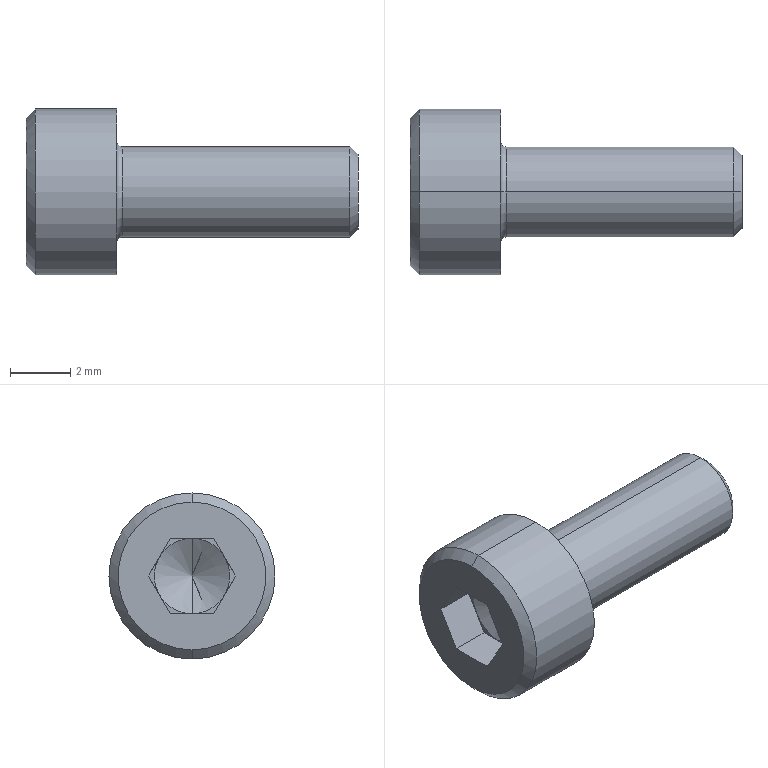Part | NX | features BREP 1 | 1 solid | 27 faces | box 11 x 5.5 x 5.5 mm | volume 118.616 mm3 | plane 15 | cone 6 | cylinder 4 | torus 2 | commonest cylinder face diameters 3 x2 5.5 x2
STEP:
#1=CARTESIAN_POINT('',(-1.7,0.,1.25));
#2=VERTEX_POINT('',#1);
#3=CARTESIAN_POINT('',(-0.9783,0.,0.));
#4=VERTEX_POINT('',#3);
#5=CARTESIAN_POINT('',(-0.9783,0.,0.));
#6=DIRECTION('',(-0.5,0.,0.866));
#7=VECTOR('',#6,1000.);
#8=LINE('',#5,#7);
#9=EDGE_CURVE('',#2,#4,#8,.F.);
#10=ORIENTED_EDGE('',*,*,#9,.T.);
#11=CARTESIAN_POINT('',(-1.7,0.,-1.25));
#12=VERTEX_POINT('',#11);
#13=CARTESIAN_POINT('',(-0.9783,0.,0.));
#14=DIRECTION('',(-0.5,0.,-0.866));
#15=VECTOR('',#14,1000.);
#16=LINE('',#13,#15);
#17=EDGE_CURVE('',#12,#4,#16,.F.);
#18=ORIENTED_EDGE('',*,*,#17,.F.);
#19=CARTESIAN_POINT('',(-1.7,-1.083,-0.625));
#20=VERTEX_POINT('',#19);
#21=CARTESIAN_POINT('',(-1.7,0.,0.));
#22=DIRECTION('',(-1.,0.,0.));
#23=DIRECTION('',(0.,0.,1.));
#24=AXIS2_PLACEMENT_3D('',#21,#22,#23);
#25=CIRCLE('',#24,1.25);
#26=EDGE_CURVE('',#12,#20,#25,.T.);
#27=ORIENTED_EDGE('',*,*,#26,.T.);
#28=CARTESIAN_POINT('',(-1.7,-1.083,0.625));
#29=VERTEX_POINT('',#28);
#30=CARTESIAN_POINT('',(-1.7,0.,0.));
#31=DIRECTION('',(-1.,0.,0.));
#32=DIRECTION('',(0.,0.,1.));
#33=AXIS2_PLACEMENT_3D('',#30,#31,#32);
#34=CIRCLE('',#33,1.25);
#35=EDGE_CURVE('',#20,#29,#34,.T.);
#36=ORIENTED_EDGE('',*,*,#35,.T.);
#37=CARTESIAN_POINT('',(-1.7,0.,0.));
#38=DIRECTION('',(-1.,0.,0.));
#39=DIRECTION('',(0.,0.,1.));
#40=AXIS2_PLACEMENT_3D('',#37,#38,#39);
#41=CIRCLE('',#40,1.25);
#42=EDGE_CURVE('',#29,#2,#41,.T.);
#43=ORIENTED_EDGE('',*,*,#42,.T.);
#44=EDGE_LOOP('',(#10,#18,#27,#36,#43));
#45=FACE_BOUND('',#44,.T.);
#46=CARTESIAN_POINT('',(-1000.978,0.,0.));
#47=DIRECTION('',(-1.,0.,0.));
#48=DIRECTION('',(0.,0.,1.));
#49=AXIS2_PLACEMENT_3D('',#46,#47,#48);
#50=CONICAL_SURFACE('',#49,1732.051,1.047);
#51=ADVANCED_FACE('',(#45),#50,.F.);
#52=CARTESIAN_POINT('',(-3.,0.,2.45));
#53=VERTEX_POINT('',#52);
#54=CARTESIAN_POINT('',(-3.,0.,-2.45));
#55=VERTEX_POINT('',#54);
#56=CARTESIAN_POINT('',(-3.,0.,0.));
#57=DIRECTION('',(-1.,0.,0.));
#58=DIRECTION('',(0.,0.,1.));
#59=AXIS2_PLACEMENT_3D('',#56,#57,#58);
#60=CIRCLE('',#59,2.45);
#61=EDGE_CURVE('',#53,#55,#60,.T.);
#62=ORIENTED_EDGE('',*,*,#61,.F.);
#63=CARTESIAN_POINT('',(-2.7,0.,2.75));
#64=VERTEX_POINT('',#63);
#65=CARTESIAN_POINT('',(-2.7,0.,2.75));
#66=DIRECTION('',(0.7071,0.,0.7071));
#67=VECTOR('',#66,1000.);
#68=LINE('',#65,#67);
#69=EDGE_CURVE('',#53,#64,#68,.T.);
#70=ORIENTED_EDGE('',*,*,#69,.T.);
#71=CARTESIAN_POINT('',(-2.7,0.,-2.75));
#72=VERTEX_POINT('',#71);
#73=CARTESIAN_POINT('',(-2.7,0.,0.));
#74=DIRECTION('',(-1.,0.,0.));
#75=DIRECTION('',(0.,0.,1.));
#76=AXIS2_PLACEMENT_3D('',#73,#74,#75);
#77=CIRCLE('',#76,2.75);
#78=EDGE_CURVE('',#64,#72,#77,.T.);
#79=ORIENTED_EDGE('',*,*,#78,.T.);
#80=CARTESIAN_POINT('',(-2.7,0.,-2.75));
#81=DIRECTION('',(0.7071,0.,-0.7071));
#82=VECTOR('',#81,1000.);
#83=LINE('',#80,#82);
#84=EDGE_CURVE('',#55,#72,#83,.T.);
#85=ORIENTED_EDGE('',*,*,#84,.F.);
#86=EDGE_LOOP('',(#62,#70,#79,#85));
#87=FACE_BOUND('',#86,.T.);
#88=CARTESIAN_POINT('',(-2.7,0.,0.));
#89=DIRECTION('',(1.,0.,0.));
#90=DIRECTION('',(0.,0.,-1.));
#91=AXIS2_PLACEMENT_3D('',#88,#89,#90);
#92=CONICAL_SURFACE('',#91,2.75,0.7854);
#93=ADVANCED_FACE('',(#87),#92,.T.);
#94=CARTESIAN_POINT('',(0.,0.,2.75));
#95=VERTEX_POINT('',#94);
#96=CARTESIAN_POINT('',(0.,0.,-2.75));
#97=VERTEX_POINT('',#96);
#98=CARTESIAN_POINT('',(0.,0.,0.));
#99=DIRECTION('',(-1.,0.,0.));
#100=DIRECTION('',(0.,0.,1.));
#101=AXIS2_PLACEMENT_3D('',#98,#99,#100);
#102=CIRCLE('',#101,2.75);
#103=EDGE_CURVE('',#95,#97,#102,.T.);
#104=ORIENTED_EDGE('',*,*,#103,.T.);
#105=CARTESIAN_POINT('',(8.,0.,-2.75));
#106=DIRECTION('',(-1.,0.,0.));
#107=VECTOR('',#106,1000.);
#108=LINE('',#105,#107);
#109=EDGE_CURVE('',#72,#97,#108,.F.);
#110=ORIENTED_EDGE('',*,*,#109,.F.);
#111=ORIENTED_EDGE('',*,*,#78,.F.);
#112=CARTESIAN_POINT('',(8.,0.,2.75));
#113=DIRECTION('',(-1.,0.,0.));
#114=VECTOR('',#113,1000.);
#115=LINE('',#112,#114);
#116=EDGE_CURVE('',#64,#95,#115,.F.);
#117=ORIENTED_EDGE('',*,*,#116,.T.);
#118=EDGE_LOOP('',(#104,#110,#111,#117));
#119=FACE_BOUND('',#118,.T.);
#120=CARTESIAN_POINT('',(8.,0.,0.));
#121=DIRECTION('',(-1.,0.,0.));
#122=DIRECTION('',(0.,0.,1.));
#123=AXIS2_PLACEMENT_3D('',#120,#121,#122);
#124=CYLINDRICAL_SURFACE('',#123,2.75);
#125=ADVANCED_FACE('',(#119),#124,.T.);
#126=CARTESIAN_POINT('',(0.,0.,-1.7));
#127=VERTEX_POINT('',#126);
#128=CARTESIAN_POINT('',(0.,0.,1.7));
#129=VERTEX_POINT('',#128);
#130=CARTESIAN_POINT('',(0.,0.,0.));
#131=DIRECTION('',(-1.,0.,0.));
#132=DIRECTION('',(0.,0.,1.));
#133=AXIS2_PLACEMENT_3D('',#130,#131,#132);
#134=CIRCLE('',#133,1.7);
#135=EDGE_CURVE('',#127,#129,#134,.T.);
#136=ORIENTED_EDGE('',*,*,#135,.F.);
#137=CARTESIAN_POINT('',(0.2,0.,-1.5));
#138=VERTEX_POINT('',#137);
#139=CARTESIAN_POINT('',(0.2,0.,-1.7));
#140=DIRECTION('',(0.,1.,0.));
#141=DIRECTION('',(0.,0.,1.));
#142=AXIS2_PLACEMENT_3D('',#139,#140,#141);
#143=CIRCLE('',#142,0.2);
#144=EDGE_CURVE('',#138,#127,#143,.F.);
#145=ORIENTED_EDGE('',*,*,#144,.F.);
#146=CARTESIAN_POINT('',(0.2,0.,1.5));
#147=VERTEX_POINT('',#146);
#148=CARTESIAN_POINT('',(0.2,0.,0.));
#149=DIRECTION('',(-1.,0.,0.));
#150=DIRECTION('',(0.,0.,1.));
#151=AXIS2_PLACEMENT_3D('',#148,#149,#150);
#152=CIRCLE('',#151,1.5);
#153=EDGE_CURVE('',#138,#147,#152,.T.);
#154=ORIENTED_EDGE('',*,*,#153,.T.);
#155=CARTESIAN_POINT('',(0.2,0.,1.7));
#156=DIRECTION('',(0.,-1.,0.));
#157=DIRECTION('',(0.,0.,-1.));
#158=AXIS2_PLACEMENT_3D('',#155,#156,#157);
#159=CIRCLE('',#158,0.2);
#160=EDGE_CURVE('',#147,#129,#159,.F.);
#161=ORIENTED_EDGE('',*,*,#160,.T.);
#162=EDGE_LOOP('',(#136,#145,#154,#161));
#163=FACE_BOUND('',#162,.T.);
#164=CARTESIAN_POINT('',(0.2,0.,0.));
#165=DIRECTION('',(-1.,0.,0.));
#166=DIRECTION('',(0.,0.,1.));
#167=AXIS2_PLACEMENT_3D('',#164,#165,#166);
#168=TOROIDAL_SURFACE('',#167,1.7,0.2);
#169=ADVANCED_FACE('',(#163),#168,.F.);
#170=CARTESIAN_POINT('',(7.729,0.,1.5));
#171=VERTEX_POINT('',#170);
#172=CARTESIAN_POINT('',(7.729,0.,-1.5));
#173=VERTEX_POINT('',#172);
#174=CARTESIAN_POINT('',(7.729,0.,0.));
#175=DIRECTION('',(-1.,0.,0.));
#176=DIRECTION('',(0.,0.,1.));
#177=AXIS2_PLACEMENT_3D('',#174,#175,#176);
#178=CIRCLE('',#177,1.5);
#179=EDGE_CURVE('',#171,#173,#178,.T.);
#180=ORIENTED_EDGE('',*,*,#179,.T.);
#181=CARTESIAN_POINT('',(8.,0.,-1.5));
#182=DIRECTION('',(-1.,0.,0.));
#183=VECTOR('',#182,1000.);
#184=LINE('',#181,#183);
#185=EDGE_CURVE('',#138,#173,#184,.F.);
#186=ORIENTED_EDGE('',*,*,#185,.F.);
#187=CARTESIAN_POINT('',(0.2,0.,0.));
#188=DIRECTION('',(-1.,0.,0.));
#189=DIRECTION('',(0.,0.,1.));
#190=AXIS2_PLACEMENT_3D('',#187,#188,#189);
#191=CIRCLE('',#190,1.5);
#192=EDGE_CURVE('',#147,#138,#191,.T.);
#193=ORIENTED_EDGE('',*,*,#192,.F.);
#194=CARTESIAN_POINT('',(8.,0.,1.5));
#195=DIRECTION('',(-1.,0.,0.));
#196=VECTOR('',#195,1000.);
#197=LINE('',#194,#196);
#198=EDGE_CURVE('',#147,#171,#197,.F.);
#199=ORIENTED_EDGE('',*,*,#198,.T.);
#200=EDGE_LOOP('',(#180,#186,#193,#199));
#201=FACE_BOUND('',#200,.T.);
#202=CARTESIAN_POINT('',(8.,0.,0.));
#203=DIRECTION('',(-1.,0.,0.));
#204=DIRECTION('',(0.,0.,1.));
#205=AXIS2_PLACEMENT_3D('',#202,#203,#204);
#206=CYLINDRICAL_SURFACE('',#205,1.5);
#207=ADVANCED_FACE('',(#201),#206,.T.);
#208=CARTESIAN_POINT('',(8.,0.,1.23));
#209=VERTEX_POINT('',#208);
#210=CARTESIAN_POINT('',(8.,0.,-1.23));
#211=VERTEX_POINT('',#210);
#212=CARTESIAN_POINT('',(8.,0.,0.));
#213=DIRECTION('',(-1.,0.,0.));
#214=DIRECTION('',(0.,0.,1.));
#215=AXIS2_PLACEMENT_3D('',#212,#213,#214);
#216=CIRCLE('',#215,1.23);
#217=EDGE_CURVE('',#209,#211,#216,.T.);
#218=ORIENTED_EDGE('',*,*,#217,.T.);
#219=CARTESIAN_POINT('',(8.,0.,-1.23));
#220=DIRECTION('',(-0.7071,0.,-0.7071));
#221=VECTOR('',#220,1000.);
#222=LINE('',#219,#221);
#223=EDGE_CURVE('',#173,#211,#222,.F.);
#224=ORIENTED_EDGE('',*,*,#223,.F.);
#225=ORIENTED_EDGE('',*,*,#179,.F.);
#226=CARTESIAN_POINT('',(8.,0.,1.23));
#227=DIRECTION('',(-0.7071,0.,0.7071));
#228=VECTOR('',#227,1000.);
#229=LINE('',#226,#228);
#230=EDGE_CURVE('',#171,#209,#229,.F.);
#231=ORIENTED_EDGE('',*,*,#230,.T.);
#232=EDGE_LOOP('',(#218,#224,#225,#231));
#233=FACE_BOUND('',#232,.T.);
#234=CARTESIAN_POINT('',(8.,0.,0.));
#235=DIRECTION('',(-1.,0.,0.));
#236=DIRECTION('',(0.,0.,1.));
#237=AXIS2_PLACEMENT_3D('',#234,#235,#236);
#238=CONICAL_SURFACE('',#237,1.23,0.7854);
#239=ADVANCED_FACE('',(#233),#238,.T.);
#240=CARTESIAN_POINT('',(-1.7,1.083,0.625));
#241=VERTEX_POINT('',#240);
#242=CARTESIAN_POINT('',(-1.7,0.,0.));
#243=DIRECTION('',(-1.,0.,0.));
#244=DIRECTION('',(0.,0.,1.));
#245=AXIS2_PLACEMENT_3D('',#242,#243,#244);
#246=CIRCLE('',#245,1.25);
#247=EDGE_CURVE('',#2,#241,#246,.T.);
#248=ORIENTED_EDGE('',*,*,#247,.F.);
#249=CARTESIAN_POINT('',(-1.7,0.7217,1.25));
#250=VERTEX_POINT('',#249);
#251=CARTESIAN_POINT('',(-1.7,0.7217,1.25));
#252=DIRECTION('',(0.,-1.,0.));
#253=VECTOR('',#252,1000.);
#254=LINE('',#251,#253);
#255=EDGE_CURVE('',#250,#2,#254,.T.);
#256=ORIENTED_EDGE('',*,*,#255,.F.);
#257=CARTESIAN_POINT('',(-1.7,1.443,0.));
#258=DIRECTION('',(0.,-0.5,0.866));
#259=VECTOR('',#258,1000.);
#260=LINE('',#257,#259);
#261=EDGE_CURVE('',#241,#250,#260,.T.);
#262=ORIENTED_EDGE('',*,*,#261,.F.);
#263=EDGE_LOOP('',(#248,#256,#262));
#264=FACE_BOUND('',#263,.T.);
#265=CARTESIAN_POINT('',(-1.7,0.7217,1.25));
#266=DIRECTION('',(1.,0.,0.));
#267=DIRECTION('',(0.,1.,0.));
#268=AXIS2_PLACEMENT_3D('',#265,#266,#267);
#269=PLANE('',#268);
#270=ADVANCED_FACE('',(#264),#269,.F.);
#271=CARTESIAN_POINT('',(-1.7,1.083,-0.625));
#272=VERTEX_POINT('',#271);
#273=CARTESIAN_POINT('',(-1.7,0.,0.));
#274=DIRECTION('',(-1.,0.,0.));
#275=DIRECTION('',(0.,0.,1.));
#276=AXIS2_PLACEMENT_3D('',#273,#274,#275);
#277=CIRCLE('',#276,1.25);
#278=EDGE_CURVE('',#241,#272,#277,.T.);
#279=ORIENTED_EDGE('',*,*,#278,.F.);
#280=CARTESIAN_POINT('',(-1.7,1.443,0.));
#281=VERTEX_POINT('',#280);
#282=CARTESIAN_POINT('',(-1.7,1.443,0.));
#283=DIRECTION('',(0.,-0.5,0.866));
#284=VECTOR('',#283,1000.);
#285=LINE('',#282,#284);
#286=EDGE_CURVE('',#281,#241,#285,.T.);
#287=ORIENTED_EDGE('',*,*,#286,.F.);
#288=CARTESIAN_POINT('',(-1.7,0.7217,-1.25));
#289=DIRECTION('',(0.,0.5,0.866));
#290=VECTOR('',#289,1000.);
#291=LINE('',#288,#290);
#292=EDGE_CURVE('',#272,#281,#291,.T.);
#293=ORIENTED_EDGE('',*,*,#292,.F.);
#294=EDGE_LOOP('',(#279,#287,#293));
#295=FACE_BOUND('',#294,.T.);
#296=CARTESIAN_POINT('',(-1.7,0.7217,1.25));
#297=DIRECTION('',(1.,0.,0.));
#298=DIRECTION('',(0.,1.,0.));
#299=AXIS2_PLACEMENT_3D('',#296,#297,#298);
#300=PLANE('',#299);
#301=ADVANCED_FACE('',(#295),#300,.F.);
#302=CARTESIAN_POINT('',(-1.7,0.,0.));
#303=DIRECTION('',(-1.,0.,0.));
#304=DIRECTION('',(0.,0.,1.));
#305=AXIS2_PLACEMENT_3D('',#302,#303,#304);
#306=CIRCLE('',#305,1.25);
#307=EDGE_CURVE('',#272,#12,#306,.T.);
#308=ORIENTED_EDGE('',*,*,#307,.F.);
#309=CARTESIAN_POINT('',(-1.7,0.7217,-1.25));
#310=VERTEX_POINT('',#309);
#311=CARTESIAN_POINT('',(-1.7,0.7217,-1.25));
#312=DIRECTION('',(0.,0.5,0.866));
#313=VECTOR('',#312,1000.);
#314=LINE('',#311,#313);
#315=EDGE_CURVE('',#310,#272,#314,.T.);
#316=ORIENTED_EDGE('',*,*,#315,.F.);
#317=CARTESIAN_POINT('',(-1.7,-0.7217,-1.25));
#318=DIRECTION('',(0.,1.,0.));
#319=VECTOR('',#318,1000.);
#320=LINE('',#317,#319);
#321=EDGE_CURVE('',#12,#310,#320,.T.);
#322=ORIENTED_EDGE('',*,*,#321,.F.);
#323=EDGE_LOOP('',(#308,#316,#322));
#324=FACE_BOUND('',#323,.T.);
#325=CARTESIAN_POINT('',(-1.7,0.7217,1.25));
#326=DIRECTION('',(1.,0.,0.));
#327=DIRECTION('',(0.,1.,0.));
#328=AXIS2_PLACEMENT_3D('',#325,#326,#327);
#329=PLANE('',#328);
#330=ADVANCED_FACE('',(#324),#329,.F.);
#331=ORIENTED_EDGE('',*,*,#26,.F.);
#332=CARTESIAN_POINT('',(-1.7,-0.7217,-1.25));
#333=VERTEX_POINT('',#332);
#334=CARTESIAN_POINT('',(-1.7,-0.7217,-1.25));
#335=DIRECTION('',(0.,1.,0.));
#336=VECTOR('',#335,1000.);
#337=LINE('',#334,#336);
#338=EDGE_CURVE('',#333,#12,#337,.T.);
#339=ORIENTED_EDGE('',*,*,#338,.F.);
#340=CARTESIAN_POINT('',(-1.7,-1.443,0.));
#341=DIRECTION('',(0.,0.5,-0.866));
#342=VECTOR('',#341,1000.);
#343=LINE('',#340,#342);
#344=EDGE_CURVE('',#20,#333,#343,.T.);
#345=ORIENTED_EDGE('',*,*,#344,.F.);
#346=EDGE_LOOP('',(#331,#339,#345));
#347=FACE_BOUND('',#346,.T.);
#348=CARTESIAN_POINT('',(-1.7,0.7217,1.25));
#349=DIRECTION('',(1.,0.,0.));
#350=DIRECTION('',(0.,1.,0.));
#351=AXIS2_PLACEMENT_3D('',#348,#349,#350);
#352=PLANE('',#351);
#353=ADVANCED_FACE('',(#347),#352,.F.);
#354=ORIENTED_EDGE('',*,*,#35,.F.);
#355=CARTESIAN_POINT('',(-1.7,-1.443,0.));
#356=VERTEX_POINT('',#355);
#357=CARTESIAN_POINT('',(-1.7,-1.443,0.));
#358=DIRECTION('',(0.,0.5,-0.866));
#359=VECTOR('',#358,1000.);
#360=LINE('',#357,#359);
#361=EDGE_CURVE('',#356,#20,#360,.T.);
#362=ORIENTED_EDGE('',*,*,#361,.F.);
#363=CARTESIAN_POINT('',(-1.7,-0.7217,1.25));
#364=DIRECTION('',(0.,-0.5,-0.866));
#365=VECTOR('',#364,1000.);
#366=LINE('',#363,#365);
#367=EDGE_CURVE('',#29,#356,#366,.T.);
#368=ORIENTED_EDGE('',*,*,#367,.F.);
#369=EDGE_LOOP('',(#354,#362,#368));
#370=FACE_BOUND('',#369,.T.);
#371=CARTESIAN_POINT('',(-1.7,0.7217,1.25));
#372=DIRECTION('',(1.,0.,0.));
#373=DIRECTION('',(0.,1.,0.));
#374=AXIS2_PLACEMENT_3D('',#371,#372,#373);
#375=PLANE('',#374);
#376=ADVANCED_FACE('',(#370),#375,.F.);
#377=ORIENTED_EDGE('',*,*,#42,.F.);
#378=CARTESIAN_POINT('',(-1.7,-0.7217,1.25));
#379=VERTEX_POINT('',#378);
#380=CARTESIAN_POINT('',(-1.7,-0.7217,1.25));
#381=DIRECTION('',(0.,-0.5,-0.866));
#382=VECTOR('',#381,1000.);
#383=LINE('',#380,#382);
#384=EDGE_CURVE('',#379,#29,#383,.T.);
#385=ORIENTED_EDGE('',*,*,#384,.F.);
#386=CARTESIAN_POINT('',(-1.7,0.7217,1.25));
#387=DIRECTION('',(0.,-1.,0.));
#388=VECTOR('',#387,1000.);
#389=LINE('',#386,#388);
#390=EDGE_CURVE('',#2,#379,#389,.T.);
#391=ORIENTED_EDGE('',*,*,#390,.F.);
#392=EDGE_LOOP('',(#377,#385,#391));
#393=FACE_BOUND('',#392,.T.);
#394=CARTESIAN_POINT('',(-1.7,0.7217,1.25));
#395=DIRECTION('',(1.,0.,0.));
#396=DIRECTION('',(0.,1.,0.));
#397=AXIS2_PLACEMENT_3D('',#394,#395,#396);
#398=PLANE('',#397);
#399=ADVANCED_FACE('',(#393),#398,.F.);
#400=CARTESIAN_POINT('',(-3.,0.,0.));
#401=DIRECTION('',(-1.,0.,0.));
#402=DIRECTION('',(0.,0.,1.));
#403=AXIS2_PLACEMENT_3D('',#400,#401,#402);
#404=CIRCLE('',#403,2.45);
#405=EDGE_CURVE('',#55,#53,#404,.T.);
#406=ORIENTED_EDGE('',*,*,#405,.T.);
#407=ORIENTED_EDGE('',*,*,#61,.T.);
#408=EDGE_LOOP('',(#406,#407));
#409=FACE_BOUND('',#408,.T.);
#410=CARTESIAN_POINT('',(-3.,1.443,0.));
#411=VERTEX_POINT('',#410);
#412=CARTESIAN_POINT('',(-3.,0.7217,1.25));
#413=VERTEX_POINT('',#412);
#414=CARTESIAN_POINT('',(-3.,1.443,0.));
#415=DIRECTION('',(0.,-0.5,0.866));
#416=VECTOR('',#415,1000.);
#417=LINE('',#414,#416);
#418=EDGE_CURVE('',#411,#413,#417,.T.);
#419=ORIENTED_EDGE('',*,*,#418,.T.);
#420=CARTESIAN_POINT('',(-3.,-0.7217,1.25));
#421=VERTEX_POINT('',#420);
#422=CARTESIAN_POINT('',(-3.,0.7217,1.25));
#423=DIRECTION('',(0.,-1.,0.));
#424=VECTOR('',#423,1000.);
#425=LINE('',#422,#424);
#426=EDGE_CURVE('',#413,#421,#425,.T.);
#427=ORIENTED_EDGE('',*,*,#426,.T.);
#428=CARTESIAN_POINT('',(-3.,-1.443,0.));
#429=VERTEX_POINT('',#428);
#430=CARTESIAN_POINT('',(-3.,-0.7217,1.25));
#431=DIRECTION('',(0.,-0.5,-0.866));
#432=VECTOR('',#431,1000.);
#433=LINE('',#430,#432);
#434=EDGE_CURVE('',#421,#429,#433,.T.);
#435=ORIENTED_EDGE('',*,*,#434,.T.);
#436=CARTESIAN_POINT('',(-3.,-0.7217,-1.25));
#437=VERTEX_POINT('',#436);
#438=CARTESIAN_POINT('',(-3.,-1.443,0.));
#439=DIRECTION('',(0.,0.5,-0.866));
#440=VECTOR('',#439,1000.);
#441=LINE('',#438,#440);
#442=EDGE_CURVE('',#429,#437,#441,.T.);
#443=ORIENTED_EDGE('',*,*,#442,.T.);
#444=CARTESIAN_POINT('',(-3.,0.7217,-1.25));
#445=VERTEX_POINT('',#444);
#446=CARTESIAN_POINT('',(-3.,-0.7217,-1.25));
#447=DIRECTION('',(0.,1.,0.));
#448=VECTOR('',#447,1000.);
#449=LINE('',#446,#448);
#450=EDGE_CURVE('',#437,#445,#449,.T.);
#451=ORIENTED_EDGE('',*,*,#450,.T.);
#452=CARTESIAN_POINT('',(-3.,0.7217,-1.25));
#453=DIRECTION('',(0.,0.5,0.866));
#454=VECTOR('',#453,1000.);
#455=LINE('',#452,#454);
#456=EDGE_CURVE('',#445,#411,#455,.T.);
#457=ORIENTED_EDGE('',*,*,#456,.T.);
#458=EDGE_LOOP('',(#419,#427,#435,#443,#451,#457));
#459=FACE_BOUND('',#458,.T.);
#460=CARTESIAN_POINT('',(-3.,0.,0.));
#461=DIRECTION('',(1.,0.,0.));
#462=DIRECTION('',(0.,1.,0.));
#463=AXIS2_PLACEMENT_3D('',#460,#461,#462);
#464=PLANE('',#463);
#465=ADVANCED_FACE('',(#409,#459),#464,.F.);
#466=ORIENTED_EDGE('',*,*,#217,.F.);
#467=CARTESIAN_POINT('',(8.,0.,0.));
#468=DIRECTION('',(-1.,0.,0.));
#469=DIRECTION('',(0.,0.,1.));
#470=AXIS2_PLACEMENT_3D('',#467,#468,#469);
#471=CIRCLE('',#470,1.23);
#472=EDGE_CURVE('',#211,#209,#471,.T.);
#473=ORIENTED_EDGE('',*,*,#472,.F.);
#474=EDGE_LOOP('',(#466,#473));
#475=FACE_BOUND('',#474,.T.);
#476=CARTESIAN_POINT('',(8.,1.23,0.));
#477=DIRECTION('',(-1.,0.,0.));
#478=DIRECTION('',(0.,0.,1.));
#479=AXIS2_PLACEMENT_3D('',#476,#477,#478);
#480=PLANE('',#479);
#481=ADVANCED_FACE('',(#475),#480,.F.);
#482=ORIENTED_EDGE('',*,*,#223,.T.);
#483=ORIENTED_EDGE('',*,*,#472,.T.);
#484=ORIENTED_EDGE('',*,*,#230,.F.);
#485=CARTESIAN_POINT('',(7.729,0.,0.));
#486=DIRECTION('',(-1.,0.,0.));
#487=DIRECTION('',(0.,0.,1.));
#488=AXIS2_PLACEMENT_3D('',#485,#486,#487);
#489=CIRCLE('',#488,1.5);
#490=EDGE_CURVE('',#173,#171,#489,.T.);
#491=ORIENTED_EDGE('',*,*,#490,.F.);
#492=EDGE_LOOP('',(#482,#483,#484,#491));
#493=FACE_BOUND('',#492,.T.);
#494=CARTESIAN_POINT('',(8.,0.,0.));
#495=DIRECTION('',(-1.,0.,0.));
#496=DIRECTION('',(0.,0.,1.));
#497=AXIS2_PLACEMENT_3D('',#494,#495,#496);
#498=CONICAL_SURFACE('',#497,1.23,0.7854);
#499=ADVANCED_FACE('',(#493),#498,.T.);
#500=ORIENTED_EDGE('',*,*,#185,.T.);
#501=ORIENTED_EDGE('',*,*,#490,.T.);
#502=ORIENTED_EDGE('',*,*,#198,.F.);
#503=ORIENTED_EDGE('',*,*,#153,.F.);
#504=EDGE_LOOP('',(#500,#501,#502,#503));
#505=FACE_BOUND('',#504,.T.);
#506=CARTESIAN_POINT('',(8.,0.,0.));
#507=DIRECTION('',(-1.,0.,0.));
#508=DIRECTION('',(0.,0.,1.));
#509=AXIS2_PLACEMENT_3D('',#506,#507,#508);
#510=CYLINDRICAL_SURFACE('',#509,1.5);
#511=ADVANCED_FACE('',(#505),#510,.T.);
#512=ORIENTED_EDGE('',*,*,#144,.T.);
#513=CARTESIAN_POINT('',(0.,0.,0.));
#514=DIRECTION('',(-1.,0.,0.));
#515=DIRECTION('',(0.,0.,1.));
#516=AXIS2_PLACEMENT_3D('',#513,#514,#515);
#517=CIRCLE('',#516,1.7);
#518=EDGE_CURVE('',#129,#127,#517,.T.);
#519=ORIENTED_EDGE('',*,*,#518,.F.);
#520=ORIENTED_EDGE('',*,*,#160,.F.);
#521=ORIENTED_EDGE('',*,*,#192,.T.);
#522=EDGE_LOOP('',(#512,#519,#520,#521));
#523=FACE_BOUND('',#522,.T.);
#524=CARTESIAN_POINT('',(0.2,0.,0.));
#525=DIRECTION('',(-1.,0.,0.));
#526=DIRECTION('',(0.,0.,1.));
#527=AXIS2_PLACEMENT_3D('',#524,#525,#526);
#528=TOROIDAL_SURFACE('',#527,1.7,0.2);
#529=ADVANCED_FACE('',(#523),#528,.F.);
#530=ORIENTED_EDGE('',*,*,#103,.F.);
#531=CARTESIAN_POINT('',(0.,0.,0.));
#532=DIRECTION('',(-1.,0.,0.));
#533=DIRECTION('',(0.,0.,1.));
#534=AXIS2_PLACEMENT_3D('',#531,#532,#533);
#535=CIRCLE('',#534,2.75);
#536=EDGE_CURVE('',#97,#95,#535,.T.);
#537=ORIENTED_EDGE('',*,*,#536,.F.);
#538=EDGE_LOOP('',(#530,#537));
#539=FACE_BOUND('',#538,.T.);
#540=ORIENTED_EDGE('',*,*,#518,.T.);
#541=ORIENTED_EDGE('',*,*,#135,.T.);
#542=EDGE_LOOP('',(#540,#541));
#543=FACE_BOUND('',#542,.T.);
#544=CARTESIAN_POINT('',(0.,2.75,0.));
#545=DIRECTION('',(-1.,0.,0.));
#546=DIRECTION('',(0.,0.,1.));
#547=AXIS2_PLACEMENT_3D('',#544,#545,#546);
#548=PLANE('',#547);
#549=ADVANCED_FACE('',(#539,#543),#548,.F.);
#550=ORIENTED_EDGE('',*,*,#109,.T.);
#551=ORIENTED_EDGE('',*,*,#536,.T.);
#552=ORIENTED_EDGE('',*,*,#116,.F.);
#553=CARTESIAN_POINT('',(-2.7,0.,0.));
#554=DIRECTION('',(-1.,0.,0.));
#555=DIRECTION('',(0.,0.,1.));
#556=AXIS2_PLACEMENT_3D('',#553,#554,#555);
#557=CIRCLE('',#556,2.75);
#558=EDGE_CURVE('',#72,#64,#557,.T.);
#559=ORIENTED_EDGE('',*,*,#558,.F.);
#560=EDGE_LOOP('',(#550,#551,#552,#559));
#561=FACE_BOUND('',#560,.T.);
#562=CARTESIAN_POINT('',(8.,0.,0.));
#563=DIRECTION('',(-1.,0.,0.));
#564=DIRECTION('',(0.,0.,1.));
#565=AXIS2_PLACEMENT_3D('',#562,#563,#564);
#566=CYLINDRICAL_SURFACE('',#565,2.75);
#567=ADVANCED_FACE('',(#561),#566,.T.);
#568=ORIENTED_EDGE('',*,*,#69,.F.);
#569=ORIENTED_EDGE('',*,*,#405,.F.);
#570=ORIENTED_EDGE('',*,*,#84,.T.);
#571=ORIENTED_EDGE('',*,*,#558,.T.);
#572=EDGE_LOOP('',(#568,#569,#570,#571));
#573=FACE_BOUND('',#572,.T.);
#574=CARTESIAN_POINT('',(-2.7,0.,0.));
#575=DIRECTION('',(1.,0.,0.));
#576=DIRECTION('',(0.,0.,-1.));
#577=AXIS2_PLACEMENT_3D('',#574,#575,#576);
#578=CONICAL_SURFACE('',#577,2.75,0.7854);
#579=ADVANCED_FACE('',(#573),#578,.T.);
#580=ORIENTED_EDGE('',*,*,#418,.F.);
#581=CARTESIAN_POINT('',(-1.7,1.443,0.));
#582=DIRECTION('',(-1.,0.,0.));
#583=VECTOR('',#582,1000.);
#584=LINE('',#581,#583);
#585=EDGE_CURVE('',#281,#411,#584,.T.);
#586=ORIENTED_EDGE('',*,*,#585,.F.);
#587=ORIENTED_EDGE('',*,*,#286,.T.);
#588=ORIENTED_EDGE('',*,*,#261,.T.);
#589=CARTESIAN_POINT('',(-1.7,0.7217,1.25));
#590=DIRECTION('',(-1.,0.,0.));
#591=VECTOR('',#590,1000.);
#592=LINE('',#589,#591);
#593=EDGE_CURVE('',#250,#413,#592,.T.);
#594=ORIENTED_EDGE('',*,*,#593,.T.);
#595=EDGE_LOOP('',(#580,#586,#587,#588,#594));
#596=FACE_BOUND('',#595,.T.);
#597=CARTESIAN_POINT('',(-1.7,1.443,0.));
#598=DIRECTION('',(0.,-0.866,-0.5));
#599=DIRECTION('',(0.,0.5,-0.866));
#600=AXIS2_PLACEMENT_3D('',#597,#598,#599);
#601=PLANE('',#600);
#602=ADVANCED_FACE('',(#596),#601,.T.);
#603=ORIENTED_EDGE('',*,*,#426,.F.);
#604=ORIENTED_EDGE('',*,*,#593,.F.);
#605=ORIENTED_EDGE('',*,*,#255,.T.);
#606=ORIENTED_EDGE('',*,*,#390,.T.);
#607=CARTESIAN_POINT('',(-1.7,-0.7217,1.25));
#608=DIRECTION('',(-1.,0.,0.));
#609=VECTOR('',#608,1000.);
#610=LINE('',#607,#609);
#611=EDGE_CURVE('',#379,#421,#610,.T.);
#612=ORIENTED_EDGE('',*,*,#611,.T.);
#613=EDGE_LOOP('',(#603,#604,#605,#606,#612));
#614=FACE_BOUND('',#613,.T.);
#615=CARTESIAN_POINT('',(-1.7,0.7217,1.25));
#616=DIRECTION('',(0.,0.,-1.));
#617=DIRECTION('',(0.,-1.,0.));
#618=AXIS2_PLACEMENT_3D('',#615,#616,#617);
#619=PLANE('',#618);
#620=ADVANCED_FACE('',(#614),#619,.T.);
#621=ORIENTED_EDGE('',*,*,#434,.F.);
#622=ORIENTED_EDGE('',*,*,#611,.F.);
#623=ORIENTED_EDGE('',*,*,#384,.T.);
#624=ORIENTED_EDGE('',*,*,#367,.T.);
#625=CARTESIAN_POINT('',(-1.7,-1.443,0.));
#626=DIRECTION('',(-1.,0.,0.));
#627=VECTOR('',#626,1000.);
#628=LINE('',#625,#627);
#629=EDGE_CURVE('',#356,#429,#628,.T.);
#630=ORIENTED_EDGE('',*,*,#629,.T.);
#631=EDGE_LOOP('',(#621,#622,#623,#624,#630));
#632=FACE_BOUND('',#631,.T.);
#633=CARTESIAN_POINT('',(-1.7,-0.7217,1.25));
#634=DIRECTION('',(0.,0.866,-0.5));
#635=DIRECTION('',(-1.,0.,0.));
#636=AXIS2_PLACEMENT_3D('',#633,#634,#635);
#637=PLANE('',#636);
#638=ADVANCED_FACE('',(#632),#637,.T.);
#639=ORIENTED_EDGE('',*,*,#442,.F.);
#640=ORIENTED_EDGE('',*,*,#629,.F.);
#641=ORIENTED_EDGE('',*,*,#361,.T.);
#642=ORIENTED_EDGE('',*,*,#344,.T.);
#643=CARTESIAN_POINT('',(-1.7,-0.7217,-1.25));
#644=DIRECTION('',(-1.,0.,0.));
#645=VECTOR('',#644,1000.);
#646=LINE('',#643,#645);
#647=EDGE_CURVE('',#333,#437,#646,.T.);
#648=ORIENTED_EDGE('',*,*,#647,.T.);
#649=EDGE_LOOP('',(#639,#640,#641,#642,#648));
#650=FACE_BOUND('',#649,.T.);
#651=CARTESIAN_POINT('',(-1.7,-1.443,0.));
#652=DIRECTION('',(0.,0.866,0.5));
#653=DIRECTION('',(1.,0.,0.));
#654=AXIS2_PLACEMENT_3D('',#651,#652,#653);
#655=PLANE('',#654);
#656=ADVANCED_FACE('',(#650),#655,.T.);
#657=ORIENTED_EDGE('',*,*,#450,.F.);
#658=ORIENTED_EDGE('',*,*,#647,.F.);
#659=ORIENTED_EDGE('',*,*,#338,.T.);
#660=ORIENTED_EDGE('',*,*,#321,.T.);
#661=CARTESIAN_POINT('',(-1.7,0.7217,-1.25));
#662=DIRECTION('',(-1.,0.,0.));
#663=VECTOR('',#662,1000.);
#664=LINE('',#661,#663);
#665=EDGE_CURVE('',#310,#445,#664,.T.);
#666=ORIENTED_EDGE('',*,*,#665,.T.);
#667=EDGE_LOOP('',(#657,#658,#659,#660,#666));
#668=FACE_BOUND('',#667,.T.);
#669=CARTESIAN_POINT('',(-1.7,-0.7217,-1.25));
#670=DIRECTION('',(0.,0.,1.));
#671=DIRECTION('',(1.,0.,0.));
#672=AXIS2_PLACEMENT_3D('',#669,#670,#671);
#673=PLANE('',#672);
#674=ADVANCED_FACE('',(#668),#673,.T.);
#675=ORIENTED_EDGE('',*,*,#456,.F.);
#676=ORIENTED_EDGE('',*,*,#665,.F.);
#677=ORIENTED_EDGE('',*,*,#315,.T.);
#678=ORIENTED_EDGE('',*,*,#292,.T.);
#679=ORIENTED_EDGE('',*,*,#585,.T.);
#680=EDGE_LOOP('',(#675,#676,#677,#678,#679));
#681=FACE_BOUND('',#680,.T.);
#682=CARTESIAN_POINT('',(-1.7,0.7217,-1.25));
#683=DIRECTION('',(0.,-0.866,0.5));
#684=DIRECTION('',(-1.,0.,0.));
#685=AXIS2_PLACEMENT_3D('',#682,#683,#684);
#686=PLANE('',#685);
#687=ADVANCED_FACE('',(#681),#686,.T.);
#688=ORIENTED_EDGE('',*,*,#17,.T.);
#689=ORIENTED_EDGE('',*,*,#9,.F.);
#690=ORIENTED_EDGE('',*,*,#247,.T.);
#691=ORIENTED_EDGE('',*,*,#278,.T.);
#692=ORIENTED_EDGE('',*,*,#307,.T.);
#693=EDGE_LOOP('',(#688,#689,#690,#691,#692));
#694=FACE_BOUND('',#693,.T.);
#695=CARTESIAN_POINT('',(-1000.978,0.,0.));
#696=DIRECTION('',(-1.,0.,0.));
#697=DIRECTION('',(0.,0.,1.));
#698=AXIS2_PLACEMENT_3D('',#695,#696,#697);
#699=CONICAL_SURFACE('',#698,1732.051,1.047);
#700=ADVANCED_FACE('',(#694),#699,.F.);
#701=CLOSED_SHELL('',(#51,#93,#125,#169,#207,#239,#270,#301,#330,#353,#376,#399,#465,#481,#499,#511,#529,#549,#567,#579,#602,#620,#638,#656,#674,#687,#700));
#702=MANIFOLD_SOLID_BREP('',#701);
#703=(LENGTH_UNIT()NAMED_UNIT(*)SI_UNIT(.MILLI.,.METRE.));
#704=UNCERTAINTY_MEASURE_WITH_UNIT(LENGTH_MEASURE(0.00001),#703,'','');
#705=(NAMED_UNIT(*)PLANE_ANGLE_UNIT()SI_UNIT($,.RADIAN.));
#706=(NAMED_UNIT(*)SI_UNIT($,.STERADIAN.)SOLID_ANGLE_UNIT());
#707=(GEOMETRIC_REPRESENTATION_CONTEXT(3)GLOBAL_UNCERTAINTY_ASSIGNED_CONTEXT((#704))GLOBAL_UNIT_ASSIGNED_CONTEXT((#703,#705,#706))REPRESENTATION_CONTEXT('',''));
#708=ADVANCED_BREP_SHAPE_REPRESENTATION('',(#702),#707);